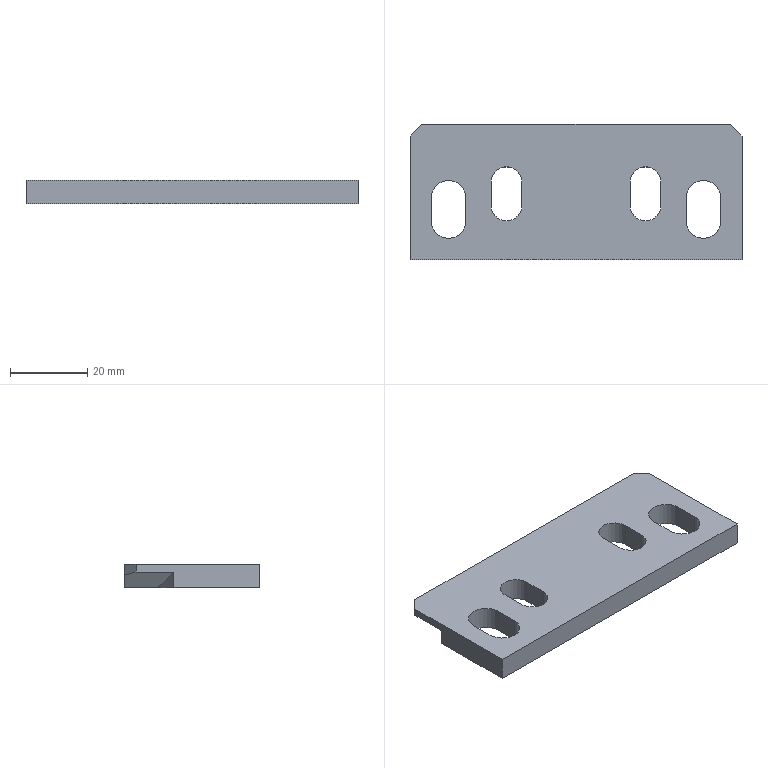Part | STEP file | gslz 2016.10.28-13_id718_x_t | 1 solid | 29 faces | box 86 x 35 x 6 mm | volume 14943 mm3 | plane 21 | cylinder 8 | commonest cylinder face diameters 8 x4 9 x4